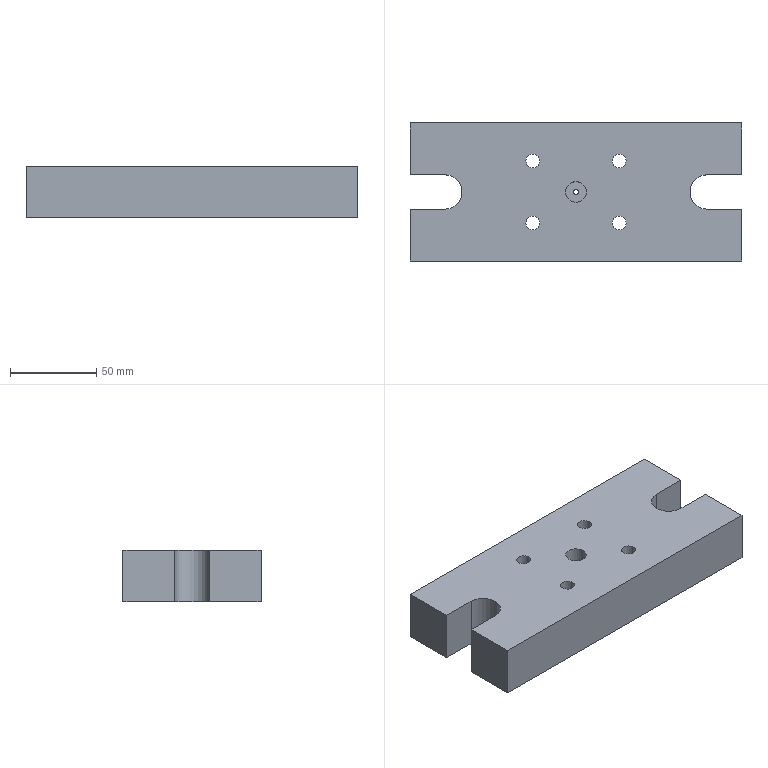Part | NX | features DATUM_CSYS 5, EXTRUDE 4, SKETCH 4 | 1 solid | 25 faces | box 192 x 80 x 30 mm | volume 417369 mm3 | plane 15 | cylinder 10 | commonest cylinder face diameters 8 x4 12 x3 20 x2 3 x1
STEP:
#1=CARTESIAN_POINT('',(-96.,-10.,0.));
#2=VERTEX_POINT('',#1);
#3=CARTESIAN_POINT('',(-96.,-40.,0.));
#4=VERTEX_POINT('',#3);
#5=CARTESIAN_POINT('',(-96.,-10.,0.));
#6=DIRECTION('',(0.,-1.,0.));
#7=VECTOR('',#6,1000.);
#8=LINE('',#5,#7);
#9=EDGE_CURVE('',#2,#4,#8,.T.);
#10=ORIENTED_EDGE('',*,*,#9,.T.);
#11=CARTESIAN_POINT('',(-96.,-40.,30.));
#12=VERTEX_POINT('',#11);
#13=CARTESIAN_POINT('',(-96.,-40.,30.));
#14=DIRECTION('',(0.,0.,-1.));
#15=VECTOR('',#14,1000.);
#16=LINE('',#13,#15);
#17=EDGE_CURVE('',#12,#4,#16,.T.);
#18=ORIENTED_EDGE('',*,*,#17,.F.);
#19=CARTESIAN_POINT('',(-96.,-10.,30.));
#20=VERTEX_POINT('',#19);
#21=CARTESIAN_POINT('',(-96.,-10.,30.));
#22=DIRECTION('',(0.,-1.,0.));
#23=VECTOR('',#22,1000.);
#24=LINE('',#21,#23);
#25=EDGE_CURVE('',#20,#12,#24,.T.);
#26=ORIENTED_EDGE('',*,*,#25,.F.);
#27=CARTESIAN_POINT('',(-96.,-10.,30.));
#28=DIRECTION('',(0.,0.,-1.));
#29=VECTOR('',#28,1000.);
#30=LINE('',#27,#29);
#31=EDGE_CURVE('',#20,#2,#30,.T.);
#32=ORIENTED_EDGE('',*,*,#31,.T.);
#33=EDGE_LOOP('',(#10,#18,#26,#32));
#34=FACE_BOUND('',#33,.T.);
#35=CARTESIAN_POINT('',(-96.,-10.,30.));
#36=DIRECTION('',(1.,0.,0.));
#37=DIRECTION('',(0.,0.,-1.));
#38=AXIS2_PLACEMENT_3D('',#35,#36,#37);
#39=PLANE('',#38);
#40=ADVANCED_FACE('',(#34),#39,.F.);
#41=CARTESIAN_POINT('',(96.,-40.,0.));
#42=VERTEX_POINT('',#41);
#43=CARTESIAN_POINT('',(-96.,-40.,0.));
#44=DIRECTION('',(1.,0.,0.));
#45=VECTOR('',#44,1000.);
#46=LINE('',#43,#45);
#47=EDGE_CURVE('',#4,#42,#46,.T.);
#48=ORIENTED_EDGE('',*,*,#47,.T.);
#49=CARTESIAN_POINT('',(96.,-40.,30.));
#50=VERTEX_POINT('',#49);
#51=CARTESIAN_POINT('',(96.,-40.,30.));
#52=DIRECTION('',(0.,0.,-1.));
#53=VECTOR('',#52,1000.);
#54=LINE('',#51,#53);
#55=EDGE_CURVE('',#50,#42,#54,.T.);
#56=ORIENTED_EDGE('',*,*,#55,.F.);
#57=CARTESIAN_POINT('',(-96.,-40.,30.));
#58=DIRECTION('',(1.,0.,0.));
#59=VECTOR('',#58,1000.);
#60=LINE('',#57,#59);
#61=EDGE_CURVE('',#12,#50,#60,.T.);
#62=ORIENTED_EDGE('',*,*,#61,.F.);
#63=ORIENTED_EDGE('',*,*,#17,.T.);
#64=EDGE_LOOP('',(#48,#56,#62,#63));
#65=FACE_BOUND('',#64,.T.);
#66=CARTESIAN_POINT('',(-96.,-40.,30.));
#67=DIRECTION('',(0.,1.,0.));
#68=DIRECTION('',(-1.,0.,0.));
#69=AXIS2_PLACEMENT_3D('',#66,#67,#68);
#70=PLANE('',#69);
#71=ADVANCED_FACE('',(#65),#70,.F.);
#72=CARTESIAN_POINT('',(96.,-10.,0.));
#73=VERTEX_POINT('',#72);
#74=CARTESIAN_POINT('',(96.,-40.,0.));
#75=DIRECTION('',(0.,1.,0.));
#76=VECTOR('',#75,1000.);
#77=LINE('',#74,#76);
#78=EDGE_CURVE('',#42,#73,#77,.T.);
#79=ORIENTED_EDGE('',*,*,#78,.T.);
#80=CARTESIAN_POINT('',(96.,-10.,30.));
#81=VERTEX_POINT('',#80);
#82=CARTESIAN_POINT('',(96.,-10.,30.));
#83=DIRECTION('',(0.,0.,-1.));
#84=VECTOR('',#83,1000.);
#85=LINE('',#82,#84);
#86=EDGE_CURVE('',#81,#73,#85,.T.);
#87=ORIENTED_EDGE('',*,*,#86,.F.);
#88=CARTESIAN_POINT('',(96.,-40.,30.));
#89=DIRECTION('',(0.,1.,0.));
#90=VECTOR('',#89,1000.);
#91=LINE('',#88,#90);
#92=EDGE_CURVE('',#50,#81,#91,.T.);
#93=ORIENTED_EDGE('',*,*,#92,.F.);
#94=ORIENTED_EDGE('',*,*,#55,.T.);
#95=EDGE_LOOP('',(#79,#87,#93,#94));
#96=FACE_BOUND('',#95,.T.);
#97=CARTESIAN_POINT('',(96.,-40.,30.));
#98=DIRECTION('',(-1.,0.,0.));
#99=DIRECTION('',(0.,0.,1.));
#100=AXIS2_PLACEMENT_3D('',#97,#98,#99);
#101=PLANE('',#100);
#102=ADVANCED_FACE('',(#96),#101,.F.);
#103=CARTESIAN_POINT('',(76.,-10.,0.));
#104=VERTEX_POINT('',#103);
#105=CARTESIAN_POINT('',(96.,-10.,0.));
#106=DIRECTION('',(-1.,0.,0.));
#107=VECTOR('',#106,1000.);
#108=LINE('',#105,#107);
#109=EDGE_CURVE('',#73,#104,#108,.T.);
#110=ORIENTED_EDGE('',*,*,#109,.T.);
#111=CARTESIAN_POINT('',(76.,-10.,30.));
#112=VERTEX_POINT('',#111);
#113=CARTESIAN_POINT('',(76.,-10.,30.));
#114=DIRECTION('',(0.,0.,-1.));
#115=VECTOR('',#114,1000.);
#116=LINE('',#113,#115);
#117=EDGE_CURVE('',#112,#104,#116,.T.);
#118=ORIENTED_EDGE('',*,*,#117,.F.);
#119=CARTESIAN_POINT('',(96.,-10.,30.));
#120=DIRECTION('',(-1.,0.,0.));
#121=VECTOR('',#120,1000.);
#122=LINE('',#119,#121);
#123=EDGE_CURVE('',#81,#112,#122,.T.);
#124=ORIENTED_EDGE('',*,*,#123,.F.);
#125=ORIENTED_EDGE('',*,*,#86,.T.);
#126=EDGE_LOOP('',(#110,#118,#124,#125));
#127=FACE_BOUND('',#126,.T.);
#128=CARTESIAN_POINT('',(96.,-10.,30.));
#129=DIRECTION('',(0.,-1.,0.));
#130=DIRECTION('',(0.,0.,-1.));
#131=AXIS2_PLACEMENT_3D('',#128,#129,#130);
#132=PLANE('',#131);
#133=ADVANCED_FACE('',(#127),#132,.F.);
#134=CARTESIAN_POINT('',(76.,10.,0.));
#135=VERTEX_POINT('',#134);
#136=CARTESIAN_POINT('',(76.,0.,0.));
#137=DIRECTION('',(0.,0.,-1.));
#138=DIRECTION('',(-1.,0.,0.));
#139=AXIS2_PLACEMENT_3D('',#136,#137,#138);
#140=CIRCLE('',#139,10.);
#141=EDGE_CURVE('',#104,#135,#140,.T.);
#142=ORIENTED_EDGE('',*,*,#141,.T.);
#143=CARTESIAN_POINT('',(76.,10.,30.));
#144=VERTEX_POINT('',#143);
#145=CARTESIAN_POINT('',(76.,10.,30.));
#146=DIRECTION('',(0.,0.,-1.));
#147=VECTOR('',#146,1000.);
#148=LINE('',#145,#147);
#149=EDGE_CURVE('',#144,#135,#148,.T.);
#150=ORIENTED_EDGE('',*,*,#149,.F.);
#151=CARTESIAN_POINT('',(76.,0.,30.));
#152=DIRECTION('',(0.,0.,-1.));
#153=DIRECTION('',(-1.,0.,0.));
#154=AXIS2_PLACEMENT_3D('',#151,#152,#153);
#155=CIRCLE('',#154,10.);
#156=EDGE_CURVE('',#112,#144,#155,.T.);
#157=ORIENTED_EDGE('',*,*,#156,.F.);
#158=ORIENTED_EDGE('',*,*,#117,.T.);
#159=EDGE_LOOP('',(#142,#150,#157,#158));
#160=FACE_BOUND('',#159,.T.);
#161=CARTESIAN_POINT('',(76.,0.,30.));
#162=DIRECTION('',(0.,0.,-1.));
#163=DIRECTION('',(-1.,0.,0.));
#164=AXIS2_PLACEMENT_3D('',#161,#162,#163);
#165=CYLINDRICAL_SURFACE('',#164,10.);
#166=ADVANCED_FACE('',(#160),#165,.F.);
#167=CARTESIAN_POINT('',(96.,10.,0.));
#168=VERTEX_POINT('',#167);
#169=CARTESIAN_POINT('',(76.,10.,0.));
#170=DIRECTION('',(1.,0.,0.));
#171=VECTOR('',#170,1000.);
#172=LINE('',#169,#171);
#173=EDGE_CURVE('',#135,#168,#172,.T.);
#174=ORIENTED_EDGE('',*,*,#173,.T.);
#175=CARTESIAN_POINT('',(96.,10.,30.));
#176=VERTEX_POINT('',#175);
#177=CARTESIAN_POINT('',(96.,10.,30.));
#178=DIRECTION('',(0.,0.,-1.));
#179=VECTOR('',#178,1000.);
#180=LINE('',#177,#179);
#181=EDGE_CURVE('',#176,#168,#180,.T.);
#182=ORIENTED_EDGE('',*,*,#181,.F.);
#183=CARTESIAN_POINT('',(76.,10.,30.));
#184=DIRECTION('',(1.,0.,0.));
#185=VECTOR('',#184,1000.);
#186=LINE('',#183,#185);
#187=EDGE_CURVE('',#144,#176,#186,.T.);
#188=ORIENTED_EDGE('',*,*,#187,.F.);
#189=ORIENTED_EDGE('',*,*,#149,.T.);
#190=EDGE_LOOP('',(#174,#182,#188,#189));
#191=FACE_BOUND('',#190,.T.);
#192=CARTESIAN_POINT('',(76.,10.,30.));
#193=DIRECTION('',(0.,1.,0.));
#194=DIRECTION('',(0.,0.,1.));
#195=AXIS2_PLACEMENT_3D('',#192,#193,#194);
#196=PLANE('',#195);
#197=ADVANCED_FACE('',(#191),#196,.F.);
#198=CARTESIAN_POINT('',(96.,40.,0.));
#199=VERTEX_POINT('',#198);
#200=CARTESIAN_POINT('',(96.,10.,0.));
#201=DIRECTION('',(0.,1.,0.));
#202=VECTOR('',#201,1000.);
#203=LINE('',#200,#202);
#204=EDGE_CURVE('',#168,#199,#203,.T.);
#205=ORIENTED_EDGE('',*,*,#204,.T.);
#206=CARTESIAN_POINT('',(96.,40.,30.));
#207=VERTEX_POINT('',#206);
#208=CARTESIAN_POINT('',(96.,40.,30.));
#209=DIRECTION('',(0.,0.,-1.));
#210=VECTOR('',#209,1000.);
#211=LINE('',#208,#210);
#212=EDGE_CURVE('',#207,#199,#211,.T.);
#213=ORIENTED_EDGE('',*,*,#212,.F.);
#214=CARTESIAN_POINT('',(96.,10.,30.));
#215=DIRECTION('',(0.,1.,0.));
#216=VECTOR('',#215,1000.);
#217=LINE('',#214,#216);
#218=EDGE_CURVE('',#176,#207,#217,.T.);
#219=ORIENTED_EDGE('',*,*,#218,.F.);
#220=ORIENTED_EDGE('',*,*,#181,.T.);
#221=EDGE_LOOP('',(#205,#213,#219,#220));
#222=FACE_BOUND('',#221,.T.);
#223=CARTESIAN_POINT('',(96.,10.,30.));
#224=DIRECTION('',(-1.,0.,0.));
#225=DIRECTION('',(0.,0.,1.));
#226=AXIS2_PLACEMENT_3D('',#223,#224,#225);
#227=PLANE('',#226);
#228=ADVANCED_FACE('',(#222),#227,.F.);
#229=CARTESIAN_POINT('',(-96.,40.,0.));
#230=VERTEX_POINT('',#229);
#231=CARTESIAN_POINT('',(96.,40.,0.));
#232=DIRECTION('',(-1.,0.,0.));
#233=VECTOR('',#232,1000.);
#234=LINE('',#231,#233);
#235=EDGE_CURVE('',#199,#230,#234,.T.);
#236=ORIENTED_EDGE('',*,*,#235,.T.);
#237=CARTESIAN_POINT('',(-96.,40.,30.));
#238=VERTEX_POINT('',#237);
#239=CARTESIAN_POINT('',(-96.,40.,30.));
#240=DIRECTION('',(0.,0.,-1.));
#241=VECTOR('',#240,1000.);
#242=LINE('',#239,#241);
#243=EDGE_CURVE('',#238,#230,#242,.T.);
#244=ORIENTED_EDGE('',*,*,#243,.F.);
#245=CARTESIAN_POINT('',(96.,40.,30.));
#246=DIRECTION('',(-1.,0.,0.));
#247=VECTOR('',#246,1000.);
#248=LINE('',#245,#247);
#249=EDGE_CURVE('',#207,#238,#248,.T.);
#250=ORIENTED_EDGE('',*,*,#249,.F.);
#251=ORIENTED_EDGE('',*,*,#212,.T.);
#252=EDGE_LOOP('',(#236,#244,#250,#251));
#253=FACE_BOUND('',#252,.T.);
#254=CARTESIAN_POINT('',(96.,40.,30.));
#255=DIRECTION('',(0.,-1.,0.));
#256=DIRECTION('',(1.,0.,0.));
#257=AXIS2_PLACEMENT_3D('',#254,#255,#256);
#258=PLANE('',#257);
#259=ADVANCED_FACE('',(#253),#258,.F.);
#260=CARTESIAN_POINT('',(-96.,10.,0.));
#261=VERTEX_POINT('',#260);
#262=CARTESIAN_POINT('',(-96.,40.,0.));
#263=DIRECTION('',(0.,-1.,0.));
#264=VECTOR('',#263,1000.);
#265=LINE('',#262,#264);
#266=EDGE_CURVE('',#230,#261,#265,.T.);
#267=ORIENTED_EDGE('',*,*,#266,.T.);
#268=CARTESIAN_POINT('',(-96.,10.,30.));
#269=VERTEX_POINT('',#268);
#270=CARTESIAN_POINT('',(-96.,10.,30.));
#271=DIRECTION('',(0.,0.,-1.));
#272=VECTOR('',#271,1000.);
#273=LINE('',#270,#272);
#274=EDGE_CURVE('',#269,#261,#273,.T.);
#275=ORIENTED_EDGE('',*,*,#274,.F.);
#276=CARTESIAN_POINT('',(-96.,40.,30.));
#277=DIRECTION('',(0.,-1.,0.));
#278=VECTOR('',#277,1000.);
#279=LINE('',#276,#278);
#280=EDGE_CURVE('',#238,#269,#279,.T.);
#281=ORIENTED_EDGE('',*,*,#280,.F.);
#282=ORIENTED_EDGE('',*,*,#243,.T.);
#283=EDGE_LOOP('',(#267,#275,#281,#282));
#284=FACE_BOUND('',#283,.T.);
#285=CARTESIAN_POINT('',(-96.,40.,30.));
#286=DIRECTION('',(1.,0.,0.));
#287=DIRECTION('',(0.,0.,-1.));
#288=AXIS2_PLACEMENT_3D('',#285,#286,#287);
#289=PLANE('',#288);
#290=ADVANCED_FACE('',(#284),#289,.F.);
#291=CARTESIAN_POINT('',(-76.,10.,0.));
#292=VERTEX_POINT('',#291);
#293=CARTESIAN_POINT('',(-96.,10.,0.));
#294=DIRECTION('',(1.,0.,0.));
#295=VECTOR('',#294,1000.);
#296=LINE('',#293,#295);
#297=EDGE_CURVE('',#261,#292,#296,.T.);
#298=ORIENTED_EDGE('',*,*,#297,.T.);
#299=CARTESIAN_POINT('',(-76.,10.,30.));
#300=VERTEX_POINT('',#299);
#301=CARTESIAN_POINT('',(-76.,10.,30.));
#302=DIRECTION('',(0.,0.,-1.));
#303=VECTOR('',#302,1000.);
#304=LINE('',#301,#303);
#305=EDGE_CURVE('',#300,#292,#304,.T.);
#306=ORIENTED_EDGE('',*,*,#305,.F.);
#307=CARTESIAN_POINT('',(-96.,10.,30.));
#308=DIRECTION('',(1.,0.,0.));
#309=VECTOR('',#308,1000.);
#310=LINE('',#307,#309);
#311=EDGE_CURVE('',#269,#300,#310,.T.);
#312=ORIENTED_EDGE('',*,*,#311,.F.);
#313=ORIENTED_EDGE('',*,*,#274,.T.);
#314=EDGE_LOOP('',(#298,#306,#312,#313));
#315=FACE_BOUND('',#314,.T.);
#316=CARTESIAN_POINT('',(-96.,10.,30.));
#317=DIRECTION('',(0.,1.,0.));
#318=DIRECTION('',(0.,0.,1.));
#319=AXIS2_PLACEMENT_3D('',#316,#317,#318);
#320=PLANE('',#319);
#321=ADVANCED_FACE('',(#315),#320,.F.);
#322=CARTESIAN_POINT('',(-76.,-10.,0.));
#323=VERTEX_POINT('',#322);
#324=CARTESIAN_POINT('',(-76.,0.,0.));
#325=DIRECTION('',(0.,0.,-1.));
#326=DIRECTION('',(1.,0.,0.));
#327=AXIS2_PLACEMENT_3D('',#324,#325,#326);
#328=CIRCLE('',#327,10.);
#329=EDGE_CURVE('',#292,#323,#328,.T.);
#330=ORIENTED_EDGE('',*,*,#329,.T.);
#331=CARTESIAN_POINT('',(-76.,-10.,30.));
#332=VERTEX_POINT('',#331);
#333=CARTESIAN_POINT('',(-76.,-10.,30.));
#334=DIRECTION('',(0.,0.,-1.));
#335=VECTOR('',#334,1000.);
#336=LINE('',#333,#335);
#337=EDGE_CURVE('',#332,#323,#336,.T.);
#338=ORIENTED_EDGE('',*,*,#337,.F.);
#339=CARTESIAN_POINT('',(-76.,0.,30.));
#340=DIRECTION('',(0.,0.,-1.));
#341=DIRECTION('',(1.,0.,0.));
#342=AXIS2_PLACEMENT_3D('',#339,#340,#341);
#343=CIRCLE('',#342,10.);
#344=EDGE_CURVE('',#300,#332,#343,.T.);
#345=ORIENTED_EDGE('',*,*,#344,.F.);
#346=ORIENTED_EDGE('',*,*,#305,.T.);
#347=EDGE_LOOP('',(#330,#338,#345,#346));
#348=FACE_BOUND('',#347,.T.);
#349=CARTESIAN_POINT('',(-76.,0.,30.));
#350=DIRECTION('',(0.,0.,-1.));
#351=DIRECTION('',(-1.,0.,0.));
#352=AXIS2_PLACEMENT_3D('',#349,#350,#351);
#353=CYLINDRICAL_SURFACE('',#352,10.);
#354=ADVANCED_FACE('',(#348),#353,.F.);
#355=CARTESIAN_POINT('',(29.,-18.,8.));
#356=VERTEX_POINT('',#355);
#357=CARTESIAN_POINT('',(25.,-18.,8.));
#358=DIRECTION('',(0.,0.,1.));
#359=DIRECTION('',(1.,0.,0.));
#360=AXIS2_PLACEMENT_3D('',#357,#358,#359);
#361=CIRCLE('',#360,4.);
#362=EDGE_CURVE('',#356,#356,#361,.T.);
#363=ORIENTED_EDGE('',*,*,#362,.F.);
#364=EDGE_LOOP('',(#363));
#365=FACE_BOUND('',#364,.T.);
#366=CARTESIAN_POINT('',(29.,-18.,30.));
#367=VERTEX_POINT('',#366);
#368=CARTESIAN_POINT('',(25.,-18.,30.));
#369=DIRECTION('',(0.,0.,1.));
#370=DIRECTION('',(1.,0.,0.));
#371=AXIS2_PLACEMENT_3D('',#368,#369,#370);
#372=CIRCLE('',#371,4.);
#373=EDGE_CURVE('',#367,#367,#372,.T.);
#374=ORIENTED_EDGE('',*,*,#373,.T.);
#375=EDGE_LOOP('',(#374));
#376=FACE_BOUND('',#375,.T.);
#377=CARTESIAN_POINT('',(25.,-18.,30.));
#378=DIRECTION('',(0.,0.,-1.));
#379=DIRECTION('',(-1.,0.,0.));
#380=AXIS2_PLACEMENT_3D('',#377,#378,#379);
#381=CYLINDRICAL_SURFACE('',#380,4.);
#382=ADVANCED_FACE('',(#365,#376),#381,.F.);
#383=CARTESIAN_POINT('',(-21.,18.,8.));
#384=VERTEX_POINT('',#383);
#385=CARTESIAN_POINT('',(-25.,18.,8.));
#386=DIRECTION('',(0.,0.,1.));
#387=DIRECTION('',(1.,0.,0.));
#388=AXIS2_PLACEMENT_3D('',#385,#386,#387);
#389=CIRCLE('',#388,4.);
#390=EDGE_CURVE('',#384,#384,#389,.T.);
#391=ORIENTED_EDGE('',*,*,#390,.F.);
#392=EDGE_LOOP('',(#391));
#393=FACE_BOUND('',#392,.T.);
#394=CARTESIAN_POINT('',(-21.,18.,30.));
#395=VERTEX_POINT('',#394);
#396=CARTESIAN_POINT('',(-25.,18.,30.));
#397=DIRECTION('',(0.,0.,1.));
#398=DIRECTION('',(1.,0.,0.));
#399=AXIS2_PLACEMENT_3D('',#396,#397,#398);
#400=CIRCLE('',#399,4.);
#401=EDGE_CURVE('',#395,#395,#400,.T.);
#402=ORIENTED_EDGE('',*,*,#401,.T.);
#403=EDGE_LOOP('',(#402));
#404=FACE_BOUND('',#403,.T.);
#405=CARTESIAN_POINT('',(-25.,18.,30.));
#406=DIRECTION('',(0.,0.,-1.));
#407=DIRECTION('',(-1.,0.,0.));
#408=AXIS2_PLACEMENT_3D('',#405,#406,#407);
#409=CYLINDRICAL_SURFACE('',#408,4.);
#410=ADVANCED_FACE('',(#393,#404),#409,.F.);
#411=CARTESIAN_POINT('',(-21.,-18.,30.));
#412=VERTEX_POINT('',#411);
#413=CARTESIAN_POINT('',(-25.,-18.,30.));
#414=DIRECTION('',(0.,0.,1.));
#415=DIRECTION('',(1.,0.,0.));
#416=AXIS2_PLACEMENT_3D('',#413,#414,#415);
#417=CIRCLE('',#416,4.);
#418=EDGE_CURVE('',#412,#412,#417,.T.);
#419=ORIENTED_EDGE('',*,*,#418,.T.);
#420=EDGE_LOOP('',(#419));
#421=FACE_BOUND('',#420,.T.);
#422=CARTESIAN_POINT('',(-21.,-18.,0.));
#423=VERTEX_POINT('',#422);
#424=CARTESIAN_POINT('',(-25.,-18.,0.));
#425=DIRECTION('',(0.,0.,1.));
#426=DIRECTION('',(1.,0.,0.));
#427=AXIS2_PLACEMENT_3D('',#424,#425,#426);
#428=CIRCLE('',#427,4.);
#429=EDGE_CURVE('',#423,#423,#428,.T.);
#430=ORIENTED_EDGE('',*,*,#429,.F.);
#431=EDGE_LOOP('',(#430));
#432=FACE_BOUND('',#431,.T.);
#433=CARTESIAN_POINT('',(-25.,-18.,30.));
#434=DIRECTION('',(0.,0.,-1.));
#435=DIRECTION('',(-1.,0.,0.));
#436=AXIS2_PLACEMENT_3D('',#433,#434,#435);
#437=CYLINDRICAL_SURFACE('',#436,4.);
#438=ADVANCED_FACE('',(#421,#432),#437,.F.);
#439=CARTESIAN_POINT('',(-76.,-10.,0.));
#440=DIRECTION('',(-1.,0.,0.));
#441=VECTOR('',#440,1000.);
#442=LINE('',#439,#441);
#443=EDGE_CURVE('',#323,#2,#442,.T.);
#444=ORIENTED_EDGE('',*,*,#443,.T.);
#445=ORIENTED_EDGE('',*,*,#31,.F.);
#446=CARTESIAN_POINT('',(-76.,-10.,30.));
#447=DIRECTION('',(-1.,0.,0.));
#448=VECTOR('',#447,1000.);
#449=LINE('',#446,#448);
#450=EDGE_CURVE('',#332,#20,#449,.T.);
#451=ORIENTED_EDGE('',*,*,#450,.F.);
#452=ORIENTED_EDGE('',*,*,#337,.T.);
#453=EDGE_LOOP('',(#444,#445,#451,#452));
#454=FACE_BOUND('',#453,.T.);
#455=CARTESIAN_POINT('',(-76.,-10.,30.));
#456=DIRECTION('',(0.,-1.,0.));
#457=DIRECTION('',(0.,0.,-1.));
#458=AXIS2_PLACEMENT_3D('',#455,#456,#457);
#459=PLANE('',#458);
#460=ADVANCED_FACE('',(#454),#459,.F.);
#461=CARTESIAN_POINT('',(29.,18.,30.));
#462=VERTEX_POINT('',#461);
#463=CARTESIAN_POINT('',(25.,18.,30.));
#464=DIRECTION('',(0.,0.,1.));
#465=DIRECTION('',(1.,0.,0.));
#466=AXIS2_PLACEMENT_3D('',#463,#464,#465);
#467=CIRCLE('',#466,4.);
#468=EDGE_CURVE('',#462,#462,#467,.T.);
#469=ORIENTED_EDGE('',*,*,#468,.T.);
#470=EDGE_LOOP('',(#469));
#471=FACE_BOUND('',#470,.T.);
#472=CARTESIAN_POINT('',(29.,18.,0.));
#473=VERTEX_POINT('',#472);
#474=CARTESIAN_POINT('',(25.,18.,0.));
#475=DIRECTION('',(0.,0.,1.));
#476=DIRECTION('',(1.,0.,0.));
#477=AXIS2_PLACEMENT_3D('',#474,#475,#476);
#478=CIRCLE('',#477,4.);
#479=EDGE_CURVE('',#473,#473,#478,.T.);
#480=ORIENTED_EDGE('',*,*,#479,.F.);
#481=EDGE_LOOP('',(#480));
#482=FACE_BOUND('',#481,.T.);
#483=CARTESIAN_POINT('',(25.,18.,30.));
#484=DIRECTION('',(0.,0.,-1.));
#485=DIRECTION('',(-1.,0.,0.));
#486=AXIS2_PLACEMENT_3D('',#483,#484,#485);
#487=CYLINDRICAL_SURFACE('',#486,4.);
#488=ADVANCED_FACE('',(#471,#482),#487,.F.);
#489=CARTESIAN_POINT('',(-6.,0.,30.));
#490=VERTEX_POINT('',#489);
#491=CARTESIAN_POINT('',(0.,0.,30.));
#492=DIRECTION('',(0.,0.,-1.));
#493=DIRECTION('',(-1.,0.,0.));
#494=AXIS2_PLACEMENT_3D('',#491,#492,#493);
#495=CIRCLE('',#494,6.);
#496=EDGE_CURVE('',#490,#490,#495,.T.);
#497=ORIENTED_EDGE('',*,*,#496,.T.);
#498=EDGE_LOOP('',(#497));
#499=FACE_BOUND('',#498,.T.);
#500=ORIENTED_EDGE('',*,*,#25,.T.);
#501=ORIENTED_EDGE('',*,*,#61,.T.);
#502=ORIENTED_EDGE('',*,*,#92,.T.);
#503=ORIENTED_EDGE('',*,*,#123,.T.);
#504=ORIENTED_EDGE('',*,*,#156,.T.);
#505=ORIENTED_EDGE('',*,*,#187,.T.);
#506=ORIENTED_EDGE('',*,*,#218,.T.);
#507=ORIENTED_EDGE('',*,*,#249,.T.);
#508=ORIENTED_EDGE('',*,*,#280,.T.);
#509=ORIENTED_EDGE('',*,*,#311,.T.);
#510=ORIENTED_EDGE('',*,*,#344,.T.);
#511=ORIENTED_EDGE('',*,*,#450,.T.);
#512=EDGE_LOOP('',(#500,#501,#502,#503,#504,#505,#506,#507,#508,#509,#510,#511));
#513=FACE_BOUND('',#512,.T.);
#514=ORIENTED_EDGE('',*,*,#418,.F.);
#515=EDGE_LOOP('',(#514));
#516=FACE_BOUND('',#515,.T.);
#517=ORIENTED_EDGE('',*,*,#401,.F.);
#518=EDGE_LOOP('',(#517));
#519=FACE_BOUND('',#518,.T.);
#520=ORIENTED_EDGE('',*,*,#373,.F.);
#521=EDGE_LOOP('',(#520));
#522=FACE_BOUND('',#521,.T.);
#523=ORIENTED_EDGE('',*,*,#468,.F.);
#524=EDGE_LOOP('',(#523));
#525=FACE_BOUND('',#524,.T.);
#526=CARTESIAN_POINT('',(76.,0.,30.));
#527=DIRECTION('',(0.,0.,-1.));
#528=DIRECTION('',(-1.,0.,0.));
#529=AXIS2_PLACEMENT_3D('',#526,#527,#528);
#530=PLANE('',#529);
#531=ADVANCED_FACE('',(#499,#513,#516,#519,#522,#525),#530,.F.);
#532=CARTESIAN_POINT('',(1.5,0.,0.));
#533=VERTEX_POINT('',#532);
#534=CARTESIAN_POINT('',(0.,0.,0.));
#535=DIRECTION('',(0.,0.,1.));
#536=DIRECTION('',(1.,0.,0.));
#537=AXIS2_PLACEMENT_3D('',#534,#535,#536);
#538=CIRCLE('',#537,1.5);
#539=EDGE_CURVE('',#533,#533,#538,.T.);
#540=ORIENTED_EDGE('',*,*,#539,.T.);
#541=EDGE_LOOP('',(#540));
#542=FACE_BOUND('',#541,.T.);
#543=CARTESIAN_POINT('',(-19.,18.,0.));
#544=VERTEX_POINT('',#543);
#545=CARTESIAN_POINT('',(-25.,18.,0.));
#546=DIRECTION('',(0.,0.,1.));
#547=DIRECTION('',(1.,0.,0.));
#548=AXIS2_PLACEMENT_3D('',#545,#546,#547);
#549=CIRCLE('',#548,6.);
#550=EDGE_CURVE('',#544,#544,#549,.T.);
#551=ORIENTED_EDGE('',*,*,#550,.T.);
#552=EDGE_LOOP('',(#551));
#553=FACE_BOUND('',#552,.T.);
#554=CARTESIAN_POINT('',(31.,-18.,0.));
#555=VERTEX_POINT('',#554);
#556=CARTESIAN_POINT('',(25.,-18.,0.));
#557=DIRECTION('',(0.,0.,1.));
#558=DIRECTION('',(1.,0.,0.));
#559=AXIS2_PLACEMENT_3D('',#556,#557,#558);
#560=CIRCLE('',#559,6.);
#561=EDGE_CURVE('',#555,#555,#560,.T.);
#562=ORIENTED_EDGE('',*,*,#561,.T.);
#563=EDGE_LOOP('',(#562));
#564=FACE_BOUND('',#563,.T.);
#565=ORIENTED_EDGE('',*,*,#9,.F.);
#566=ORIENTED_EDGE('',*,*,#443,.F.);
#567=ORIENTED_EDGE('',*,*,#329,.F.);
#568=ORIENTED_EDGE('',*,*,#297,.F.);
#569=ORIENTED_EDGE('',*,*,#266,.F.);
#570=ORIENTED_EDGE('',*,*,#235,.F.);
#571=ORIENTED_EDGE('',*,*,#204,.F.);
#572=ORIENTED_EDGE('',*,*,#173,.F.);
#573=ORIENTED_EDGE('',*,*,#141,.F.);
#574=ORIENTED_EDGE('',*,*,#109,.F.);
#575=ORIENTED_EDGE('',*,*,#78,.F.);
#576=ORIENTED_EDGE('',*,*,#47,.F.);
#577=EDGE_LOOP('',(#565,#566,#567,#568,#569,#570,#571,#572,#573,#574,#575,#576));
#578=FACE_BOUND('',#577,.T.);
#579=ORIENTED_EDGE('',*,*,#429,.T.);
#580=EDGE_LOOP('',(#579));
#581=FACE_BOUND('',#580,.T.);
#582=ORIENTED_EDGE('',*,*,#479,.T.);
#583=EDGE_LOOP('',(#582));
#584=FACE_BOUND('',#583,.T.);
#585=CARTESIAN_POINT('',(76.,0.,0.));
#586=DIRECTION('',(0.,0.,-1.));
#587=DIRECTION('',(-1.,0.,0.));
#588=AXIS2_PLACEMENT_3D('',#585,#586,#587);
#589=PLANE('',#588);
#590=ADVANCED_FACE('',(#542,#553,#564,#578,#581,#584),#589,.T.);
#591=CARTESIAN_POINT('',(31.,-18.,8.));
#592=VERTEX_POINT('',#591);
#593=CARTESIAN_POINT('',(25.,-18.,8.));
#594=DIRECTION('',(0.,0.,1.));
#595=DIRECTION('',(1.,0.,0.));
#596=AXIS2_PLACEMENT_3D('',#593,#594,#595);
#597=CIRCLE('',#596,6.);
#598=EDGE_CURVE('',#592,#592,#597,.F.);
#599=ORIENTED_EDGE('',*,*,#598,.F.);
#600=EDGE_LOOP('',(#599));
#601=FACE_BOUND('',#600,.T.);
#602=ORIENTED_EDGE('',*,*,#561,.F.);
#603=EDGE_LOOP('',(#602));
#604=FACE_BOUND('',#603,.T.);
#605=CARTESIAN_POINT('',(25.,-18.,8.));
#606=DIRECTION('',(0.,0.,-1.));
#607=DIRECTION('',(-1.,0.,0.));
#608=AXIS2_PLACEMENT_3D('',#605,#606,#607);
#609=CYLINDRICAL_SURFACE('',#608,6.);
#610=ADVANCED_FACE('',(#601,#604),#609,.F.);
#611=ORIENTED_EDGE('',*,*,#362,.T.);
#612=EDGE_LOOP('',(#611));
#613=FACE_BOUND('',#612,.T.);
#614=ORIENTED_EDGE('',*,*,#598,.T.);
#615=EDGE_LOOP('',(#614));
#616=FACE_BOUND('',#615,.T.);
#617=CARTESIAN_POINT('',(25.,-18.,8.));
#618=DIRECTION('',(0.,0.,1.));
#619=DIRECTION('',(1.,0.,0.));
#620=AXIS2_PLACEMENT_3D('',#617,#618,#619);
#621=PLANE('',#620);
#622=ADVANCED_FACE('',(#613,#616),#621,.F.);
#623=CARTESIAN_POINT('',(-19.,18.,8.));
#624=VERTEX_POINT('',#623);
#625=CARTESIAN_POINT('',(-25.,18.,8.));
#626=DIRECTION('',(0.,0.,1.));
#627=DIRECTION('',(1.,0.,0.));
#628=AXIS2_PLACEMENT_3D('',#625,#626,#627);
#629=CIRCLE('',#628,6.);
#630=EDGE_CURVE('',#624,#624,#629,.F.);
#631=ORIENTED_EDGE('',*,*,#630,.F.);
#632=EDGE_LOOP('',(#631));
#633=FACE_BOUND('',#632,.T.);
#634=ORIENTED_EDGE('',*,*,#550,.F.);
#635=EDGE_LOOP('',(#634));
#636=FACE_BOUND('',#635,.T.);
#637=CARTESIAN_POINT('',(-25.,18.,8.));
#638=DIRECTION('',(0.,0.,-1.));
#639=DIRECTION('',(-1.,0.,0.));
#640=AXIS2_PLACEMENT_3D('',#637,#638,#639);
#641=CYLINDRICAL_SURFACE('',#640,6.);
#642=ADVANCED_FACE('',(#633,#636),#641,.F.);
#643=ORIENTED_EDGE('',*,*,#390,.T.);
#644=EDGE_LOOP('',(#643));
#645=FACE_BOUND('',#644,.T.);
#646=ORIENTED_EDGE('',*,*,#630,.T.);
#647=EDGE_LOOP('',(#646));
#648=FACE_BOUND('',#647,.T.);
#649=CARTESIAN_POINT('',(-25.,18.,8.));
#650=DIRECTION('',(0.,0.,1.));
#651=DIRECTION('',(1.,0.,0.));
#652=AXIS2_PLACEMENT_3D('',#649,#650,#651);
#653=PLANE('',#652);
#654=ADVANCED_FACE('',(#645,#648),#653,.F.);
#655=CARTESIAN_POINT('',(1.5,0.,4.));
#656=VERTEX_POINT('',#655);
#657=CARTESIAN_POINT('',(0.,0.,4.));
#658=DIRECTION('',(0.,0.,1.));
#659=DIRECTION('',(1.,0.,0.));
#660=AXIS2_PLACEMENT_3D('',#657,#658,#659);
#661=CIRCLE('',#660,1.5);
#662=EDGE_CURVE('',#656,#656,#661,.F.);
#663=ORIENTED_EDGE('',*,*,#662,.F.);
#664=EDGE_LOOP('',(#663));
#665=FACE_BOUND('',#664,.T.);
#666=ORIENTED_EDGE('',*,*,#539,.F.);
#667=EDGE_LOOP('',(#666));
#668=FACE_BOUND('',#667,.T.);
#669=CARTESIAN_POINT('',(0.,0.,4.));
#670=DIRECTION('',(0.,0.,-1.));
#671=DIRECTION('',(-1.,0.,0.));
#672=AXIS2_PLACEMENT_3D('',#669,#670,#671);
#673=CYLINDRICAL_SURFACE('',#672,1.5);
#674=ADVANCED_FACE('',(#665,#668),#673,.F.);
#675=CARTESIAN_POINT('',(6.,0.,4.));
#676=VERTEX_POINT('',#675);
#677=CARTESIAN_POINT('',(0.,0.,4.));
#678=DIRECTION('',(0.,0.,-1.));
#679=DIRECTION('',(1.,0.,0.));
#680=AXIS2_PLACEMENT_3D('',#677,#678,#679);
#681=CIRCLE('',#680,6.);
#682=EDGE_CURVE('',#676,#676,#681,.F.);
#683=ORIENTED_EDGE('',*,*,#682,.F.);
#684=EDGE_LOOP('',(#683));
#685=FACE_BOUND('',#684,.T.);
#686=ORIENTED_EDGE('',*,*,#496,.F.);
#687=EDGE_LOOP('',(#686));
#688=FACE_BOUND('',#687,.T.);
#689=CARTESIAN_POINT('',(0.,0.,45.));
#690=DIRECTION('',(0.,0.,-1.));
#691=DIRECTION('',(-1.,0.,0.));
#692=AXIS2_PLACEMENT_3D('',#689,#690,#691);
#693=CYLINDRICAL_SURFACE('',#692,6.);
#694=ADVANCED_FACE('',(#685,#688),#693,.F.);
#695=ORIENTED_EDGE('',*,*,#662,.T.);
#696=EDGE_LOOP('',(#695));
#697=FACE_BOUND('',#696,.T.);
#698=ORIENTED_EDGE('',*,*,#682,.T.);
#699=EDGE_LOOP('',(#698));
#700=FACE_BOUND('',#699,.T.);
#701=CARTESIAN_POINT('',(0.,0.,4.));
#702=DIRECTION('',(0.,0.,-1.));
#703=DIRECTION('',(-1.,0.,0.));
#704=AXIS2_PLACEMENT_3D('',#701,#702,#703);
#705=PLANE('',#704);
#706=ADVANCED_FACE('',(#697,#700),#705,.F.);
#707=CLOSED_SHELL('',(#40,#71,#102,#133,#166,#197,#228,#259,#290,#321,#354,#382,#410,#438,#460,#488,#531,#590,#610,#622,#642,#654,#674,#694,#706));
#708=MANIFOLD_SOLID_BREP('',#707);
#709=(LENGTH_UNIT()NAMED_UNIT(*)SI_UNIT(.MILLI.,.METRE.));
#710=UNCERTAINTY_MEASURE_WITH_UNIT(LENGTH_MEASURE(0.00001),#709,'','');
#711=(NAMED_UNIT(*)PLANE_ANGLE_UNIT()SI_UNIT($,.RADIAN.));
#712=(NAMED_UNIT(*)SI_UNIT($,.STERADIAN.)SOLID_ANGLE_UNIT());
#713=(GEOMETRIC_REPRESENTATION_CONTEXT(3)GLOBAL_UNCERTAINTY_ASSIGNED_CONTEXT((#710))GLOBAL_UNIT_ASSIGNED_CONTEXT((#709,#711,#712))REPRESENTATION_CONTEXT('',''));
#714=ADVANCED_BREP_SHAPE_REPRESENTATION('',(#708),#713);